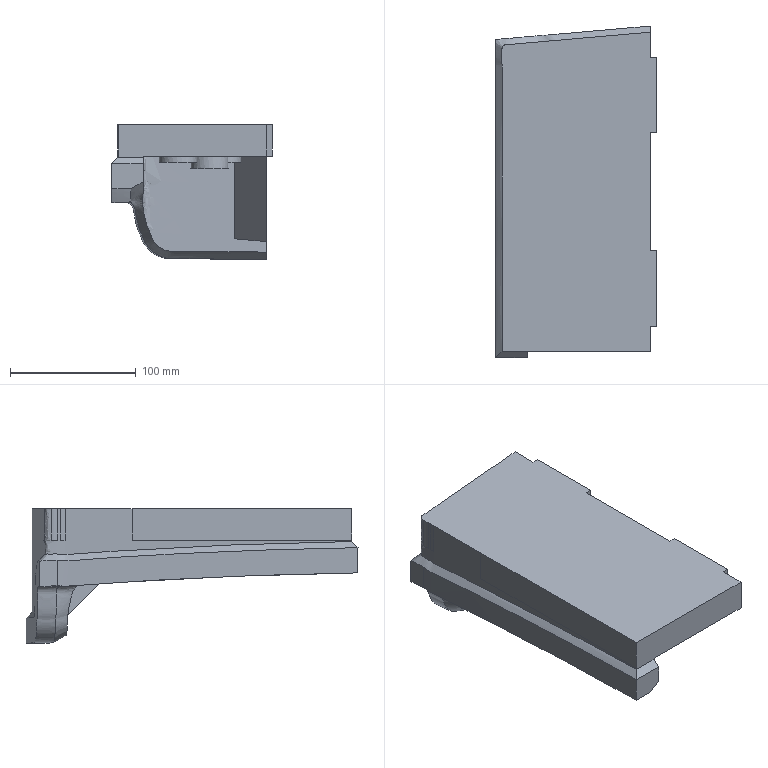Part | NX | features solid 2 | 1 solid | 41 faces | box 127.835 x 263.686 x 107.014 mm | volume 1160757 mm3 | plane 25 | spline 11 | cylinder 5 | commonest cylinder face diameters 30 x5